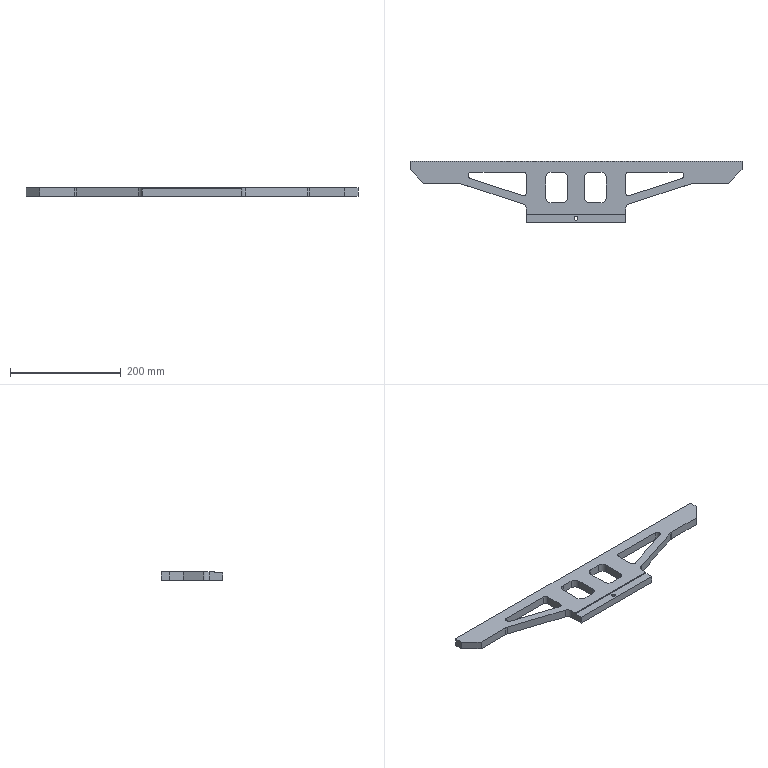Part | STEP file | 001-008-Traverse module transfer vertical plate | 1 solid | 54 faces | box 600 x 111 x 15 mm | volume 459001 mm3 | plane 32 | cylinder 22 | commonest cylinder face diameters 20 x12 10 x8 6.8 x2